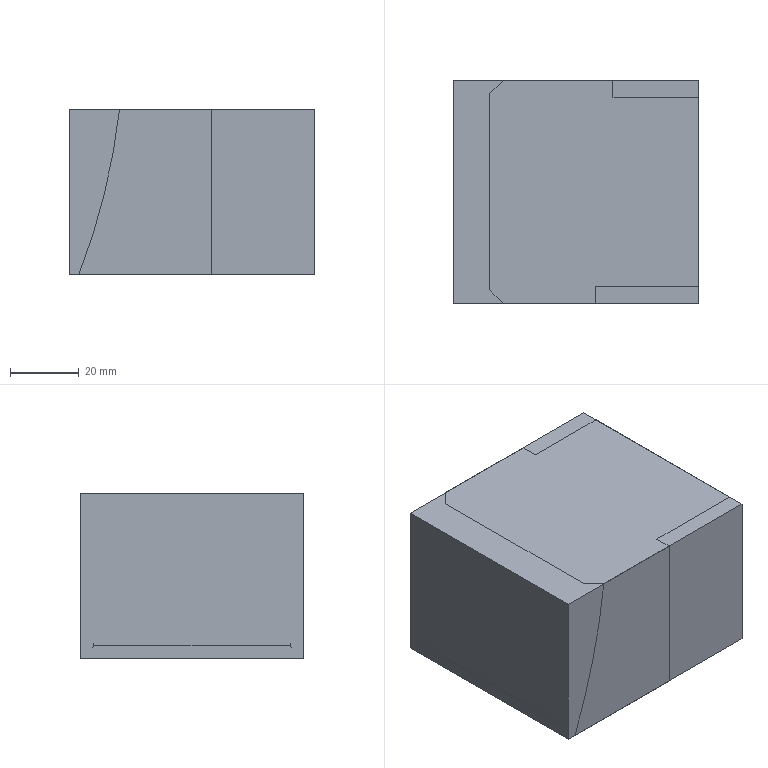Part | NX | 2 solids | 43 faces | box 71.51 x 65 x 48 mm | volume 411615 mm3 | plane 16 | cone 14 | cylinder 13 | commonest cylinder face diameters 7 x8 5 x4 379.635 x1
STEP:
#1=CARTESIAN_POINT('',(35.755,-32.5,0.));
#2=VERTEX_POINT('',#1);
#3=CARTESIAN_POINT('',(-35.755,-32.5,0.));
#4=VERTEX_POINT('',#3);
#5=CARTESIAN_POINT('',(0.,-32.5,0.));
#6=DIRECTION('',(-1.,0.,0.));
#7=VECTOR('',#6,1000.);
#8=LINE('',#5,#7);
#9=EDGE_CURVE('',#2,#4,#8,.T.);
#10=ORIENTED_EDGE('',*,*,#9,.F.);
#11=CARTESIAN_POINT('',(35.755,32.5,0.));
#12=VERTEX_POINT('',#11);
#13=CARTESIAN_POINT('',(35.755,0.,0.));
#14=DIRECTION('',(0.,-1.,0.));
#15=VECTOR('',#14,1000.);
#16=LINE('',#13,#15);
#17=EDGE_CURVE('',#12,#2,#16,.T.);
#18=ORIENTED_EDGE('',*,*,#17,.F.);
#19=CARTESIAN_POINT('',(-35.755,32.5,0.));
#20=VERTEX_POINT('',#19);
#21=CARTESIAN_POINT('',(0.,32.5,0.));
#22=DIRECTION('',(1.,0.,0.));
#23=VECTOR('',#22,1000.);
#24=LINE('',#21,#23);
#25=EDGE_CURVE('',#20,#12,#24,.T.);
#26=ORIENTED_EDGE('',*,*,#25,.F.);
#27=CARTESIAN_POINT('',(-35.755,0.,0.));
#28=DIRECTION('',(0.,1.,0.));
#29=VECTOR('',#28,1000.);
#30=LINE('',#27,#29);
#31=EDGE_CURVE('',#4,#20,#30,.T.);
#32=ORIENTED_EDGE('',*,*,#31,.F.);
#33=EDGE_LOOP('',(#10,#18,#26,#32));
#34=FACE_BOUND('',#33,.T.);
#35=CARTESIAN_POINT('',(0.,0.,0.));
#36=DIRECTION('',(0.,0.,1.));
#37=DIRECTION('',(1.,0.,0.));
#38=AXIS2_PLACEMENT_3D('',#35,#36,#37);
#39=PLANE('',#38);
#40=ADVANCED_FACE('',(#34),#39,.T.);
#41=CARTESIAN_POINT('',(35.755,-32.5,-48.));
#42=VERTEX_POINT('',#41);
#43=CARTESIAN_POINT('',(35.755,-32.5,-48.));
#44=DIRECTION('',(0.,0.,1.));
#45=VECTOR('',#44,1000.);
#46=LINE('',#43,#45);
#47=EDGE_CURVE('',#42,#2,#46,.T.);
#48=ORIENTED_EDGE('',*,*,#47,.T.);
#49=ORIENTED_EDGE('',*,*,#9,.T.);
#50=CARTESIAN_POINT('',(-35.755,-32.5,-48.));
#51=VERTEX_POINT('',#50);
#52=CARTESIAN_POINT('',(-35.755,-32.5,-48.));
#53=DIRECTION('',(0.,0.,1.));
#54=VECTOR('',#53,1000.);
#55=LINE('',#52,#54);
#56=EDGE_CURVE('',#51,#4,#55,.T.);
#57=ORIENTED_EDGE('',*,*,#56,.F.);
#58=CARTESIAN_POINT('',(0.,-32.5,-48.));
#59=DIRECTION('',(1.,0.,0.));
#60=VECTOR('',#59,1000.);
#61=LINE('',#58,#60);
#62=EDGE_CURVE('',#51,#42,#61,.T.);
#63=ORIENTED_EDGE('',*,*,#62,.T.);
#64=EDGE_LOOP('',(#48,#49,#57,#63));
#65=FACE_BOUND('',#64,.T.);
#66=CARTESIAN_POINT('',(0.,-32.5,-48.));
#67=DIRECTION('',(0.,-1.,0.));
#68=DIRECTION('',(0.,0.,-1.));
#69=AXIS2_PLACEMENT_3D('',#66,#67,#68);
#70=PLANE('',#69);
#71=ADVANCED_FACE('',(#65),#70,.T.);
#72=ORIENTED_EDGE('',*,*,#56,.T.);
#73=ORIENTED_EDGE('',*,*,#31,.T.);
#74=CARTESIAN_POINT('',(-35.755,32.5,-48.));
#75=VERTEX_POINT('',#74);
#76=CARTESIAN_POINT('',(-35.755,32.5,-48.));
#77=DIRECTION('',(0.,0.,1.));
#78=VECTOR('',#77,1000.);
#79=LINE('',#76,#78);
#80=EDGE_CURVE('',#75,#20,#79,.T.);
#81=ORIENTED_EDGE('',*,*,#80,.F.);
#82=CARTESIAN_POINT('',(-35.755,0.,-48.));
#83=DIRECTION('',(0.,-1.,0.));
#84=VECTOR('',#83,1000.);
#85=LINE('',#82,#84);
#86=EDGE_CURVE('',#75,#51,#85,.T.);
#87=ORIENTED_EDGE('',*,*,#86,.T.);
#88=EDGE_LOOP('',(#72,#73,#81,#87));
#89=FACE_BOUND('',#88,.T.);
#90=CARTESIAN_POINT('',(-35.755,0.,-48.));
#91=DIRECTION('',(-1.,0.,0.));
#92=DIRECTION('',(0.,0.,1.));
#93=AXIS2_PLACEMENT_3D('',#90,#91,#92);
#94=PLANE('',#93);
#95=ADVANCED_FACE('',(#89),#94,.T.);
#96=ORIENTED_EDGE('',*,*,#80,.T.);
#97=ORIENTED_EDGE('',*,*,#25,.T.);
#98=CARTESIAN_POINT('',(35.755,32.5,-48.));
#99=VERTEX_POINT('',#98);
#100=CARTESIAN_POINT('',(35.755,32.5,-48.));
#101=DIRECTION('',(0.,0.,1.));
#102=VECTOR('',#101,1000.);
#103=LINE('',#100,#102);
#104=EDGE_CURVE('',#99,#12,#103,.T.);
#105=ORIENTED_EDGE('',*,*,#104,.F.);
#106=CARTESIAN_POINT('',(0.,32.5,-48.));
#107=DIRECTION('',(-1.,0.,0.));
#108=VECTOR('',#107,1000.);
#109=LINE('',#106,#108);
#110=EDGE_CURVE('',#99,#75,#109,.T.);
#111=ORIENTED_EDGE('',*,*,#110,.T.);
#112=EDGE_LOOP('',(#96,#97,#105,#111));
#113=FACE_BOUND('',#112,.T.);
#114=CARTESIAN_POINT('',(0.,32.5,-48.));
#115=DIRECTION('',(0.,1.,0.));
#116=DIRECTION('',(0.,0.,1.));
#117=AXIS2_PLACEMENT_3D('',#114,#115,#116);
#118=PLANE('',#117);
#119=ADVANCED_FACE('',(#113),#118,.T.);
#120=CARTESIAN_POINT('',(35.755,0.,-48.));
#121=DIRECTION('',(0.,1.,0.));
#122=VECTOR('',#121,1000.);
#123=LINE('',#120,#122);
#124=EDGE_CURVE('',#42,#99,#123,.T.);
#125=ORIENTED_EDGE('',*,*,#124,.F.);
#126=ORIENTED_EDGE('',*,*,#62,.F.);
#127=ORIENTED_EDGE('',*,*,#86,.F.);
#128=ORIENTED_EDGE('',*,*,#110,.F.);
#129=EDGE_LOOP('',(#125,#126,#127,#128));
#130=FACE_BOUND('',#129,.T.);
#131=CARTESIAN_POINT('',(0.,0.,-48.));
#132=DIRECTION('',(0.,0.,-1.));
#133=DIRECTION('',(-1.,0.,0.));
#134=AXIS2_PLACEMENT_3D('',#131,#132,#133);
#135=PLANE('',#134);
#136=ADVANCED_FACE('',(#130),#135,.T.);
#137=ORIENTED_EDGE('',*,*,#124,.T.);
#138=ORIENTED_EDGE('',*,*,#104,.T.);
#139=ORIENTED_EDGE('',*,*,#17,.T.);
#140=ORIENTED_EDGE('',*,*,#47,.F.);
#141=EDGE_LOOP('',(#137,#138,#139,#140));
#142=FACE_BOUND('',#141,.T.);
#143=CARTESIAN_POINT('',(35.755,0.,-48.));
#144=DIRECTION('',(1.,0.,0.));
#145=DIRECTION('',(0.,0.,-1.));
#146=AXIS2_PLACEMENT_3D('',#143,#144,#145);
#147=PLANE('',#146);
#148=ADVANCED_FACE('',(#142),#147,.T.);
#149=CLOSED_SHELL('',(#40,#71,#95,#119,#136,#148));
#150=MANIFOLD_SOLID_BREP('',#149);
#151=CARTESIAN_POINT('',(23.755,-20.,-36.5));
#152=VERTEX_POINT('',#151);
#153=CARTESIAN_POINT('',(23.755,-20.,-43.5));
#154=VERTEX_POINT('',#153);
#155=CARTESIAN_POINT('',(23.755,-20.,-40.));
#156=DIRECTION('',(1.,0.,0.));
#157=DIRECTION('',(0.,0.,-1.));
#158=AXIS2_PLACEMENT_3D('',#155,#156,#157);
#159=CIRCLE('',#158,3.5);
#160=EDGE_CURVE('',#152,#154,#159,.T.);
#161=ORIENTED_EDGE('',*,*,#160,.F.);
#162=CARTESIAN_POINT('',(35.755,-20.,-36.5));
#163=VERTEX_POINT('',#162);
#164=CARTESIAN_POINT('',(35.755,-20.,-36.5));
#165=DIRECTION('',(1.,0.,0.));
#166=VECTOR('',#165,1000.);
#167=LINE('',#164,#166);
#168=EDGE_CURVE('',#163,#152,#167,.F.);
#169=ORIENTED_EDGE('',*,*,#168,.F.);
#170=CARTESIAN_POINT('',(35.755,-20.,-43.5));
#171=VERTEX_POINT('',#170);
#172=CARTESIAN_POINT('',(35.755,-20.,-40.));
#173=DIRECTION('',(1.,0.,0.));
#174=DIRECTION('',(0.,0.,-1.));
#175=AXIS2_PLACEMENT_3D('',#172,#173,#174);
#176=CIRCLE('',#175,3.5);
#177=EDGE_CURVE('',#163,#171,#176,.T.);
#178=ORIENTED_EDGE('',*,*,#177,.T.);
#179=CARTESIAN_POINT('',(35.755,-20.,-43.5));
#180=DIRECTION('',(1.,0.,0.));
#181=VECTOR('',#180,1000.);
#182=LINE('',#179,#181);
#183=EDGE_CURVE('',#171,#154,#182,.F.);
#184=ORIENTED_EDGE('',*,*,#183,.T.);
#185=EDGE_LOOP('',(#161,#169,#178,#184));
#186=FACE_BOUND('',#185,.T.);
#187=CARTESIAN_POINT('',(35.755,-20.,-40.));
#188=DIRECTION('',(1.,0.,0.));
#189=DIRECTION('',(0.,0.,1.));
#190=AXIS2_PLACEMENT_3D('',#187,#188,#189);
#191=CYLINDRICAL_SURFACE('',#190,3.5);
#192=ADVANCED_FACE('',(#186),#191,.F.);
#193=CARTESIAN_POINT('',(21.652,-20.,-40.));
#194=VERTEX_POINT('',#193);
#195=CARTESIAN_POINT('',(23.755,-20.,-43.5));
#196=DIRECTION('',(0.515,0.,-0.8572));
#197=VECTOR('',#196,1000.);
#198=LINE('',#195,#197);
#199=EDGE_CURVE('',#154,#194,#198,.F.);
#200=ORIENTED_EDGE('',*,*,#199,.T.);
#201=CARTESIAN_POINT('',(23.755,-20.,-36.5));
#202=DIRECTION('',(0.515,0.,0.8572));
#203=VECTOR('',#202,1000.);
#204=LINE('',#201,#203);
#205=EDGE_CURVE('',#152,#194,#204,.F.);
#206=ORIENTED_EDGE('',*,*,#205,.F.);
#207=ORIENTED_EDGE('',*,*,#160,.T.);
#208=EDGE_LOOP('',(#200,#206,#207));
#209=FACE_BOUND('',#208,.T.);
#210=CARTESIAN_POINT('',(23.755,-20.,-40.));
#211=DIRECTION('',(1.,0.,0.));
#212=DIRECTION('',(0.,0.,1.));
#213=AXIS2_PLACEMENT_3D('',#210,#211,#212);
#214=CONICAL_SURFACE('',#213,3.5,1.03);
#215=ADVANCED_FACE('',(#209),#214,.F.);
#216=CARTESIAN_POINT('',(23.755,-20.,-4.5));
#217=VERTEX_POINT('',#216);
#218=CARTESIAN_POINT('',(23.755,-20.,-11.5));
#219=VERTEX_POINT('',#218);
#220=CARTESIAN_POINT('',(23.755,-20.,-8.));
#221=DIRECTION('',(1.,0.,0.));
#222=DIRECTION('',(0.,0.,-1.));
#223=AXIS2_PLACEMENT_3D('',#220,#221,#222);
#224=CIRCLE('',#223,3.5);
#225=EDGE_CURVE('',#217,#219,#224,.T.);
#226=ORIENTED_EDGE('',*,*,#225,.F.);
#227=CARTESIAN_POINT('',(35.755,-20.,-4.5));
#228=VERTEX_POINT('',#227);
#229=CARTESIAN_POINT('',(35.755,-20.,-4.5));
#230=DIRECTION('',(1.,0.,0.));
#231=VECTOR('',#230,1000.);
#232=LINE('',#229,#231);
#233=EDGE_CURVE('',#228,#217,#232,.F.);
#234=ORIENTED_EDGE('',*,*,#233,.F.);
#235=CARTESIAN_POINT('',(35.755,-20.,-11.5));
#236=VERTEX_POINT('',#235);
#237=CARTESIAN_POINT('',(35.755,-20.,-8.));
#238=DIRECTION('',(1.,0.,0.));
#239=DIRECTION('',(0.,0.,-1.));
#240=AXIS2_PLACEMENT_3D('',#237,#238,#239);
#241=CIRCLE('',#240,3.5);
#242=EDGE_CURVE('',#228,#236,#241,.T.);
#243=ORIENTED_EDGE('',*,*,#242,.T.);
#244=CARTESIAN_POINT('',(35.755,-20.,-11.5));
#245=DIRECTION('',(1.,0.,0.));
#246=VECTOR('',#245,1000.);
#247=LINE('',#244,#246);
#248=EDGE_CURVE('',#236,#219,#247,.F.);
#249=ORIENTED_EDGE('',*,*,#248,.T.);
#250=EDGE_LOOP('',(#226,#234,#243,#249));
#251=FACE_BOUND('',#250,.T.);
#252=CARTESIAN_POINT('',(35.755,-20.,-8.));
#253=DIRECTION('',(1.,0.,0.));
#254=DIRECTION('',(0.,0.,1.));
#255=AXIS2_PLACEMENT_3D('',#252,#253,#254);
#256=CYLINDRICAL_SURFACE('',#255,3.5);
#257=ADVANCED_FACE('',(#251),#256,.F.);
#258=CARTESIAN_POINT('',(21.652,-20.,-8.));
#259=VERTEX_POINT('',#258);
#260=CARTESIAN_POINT('',(23.755,-20.,-11.5));
#261=DIRECTION('',(0.515,0.,-0.8572));
#262=VECTOR('',#261,1000.);
#263=LINE('',#260,#262);
#264=EDGE_CURVE('',#219,#259,#263,.F.);
#265=ORIENTED_EDGE('',*,*,#264,.T.);
#266=CARTESIAN_POINT('',(23.755,-20.,-4.5));
#267=DIRECTION('',(0.515,0.,0.8572));
#268=VECTOR('',#267,1000.);
#269=LINE('',#266,#268);
#270=EDGE_CURVE('',#217,#259,#269,.F.);
#271=ORIENTED_EDGE('',*,*,#270,.F.);
#272=ORIENTED_EDGE('',*,*,#225,.T.);
#273=EDGE_LOOP('',(#265,#271,#272));
#274=FACE_BOUND('',#273,.T.);
#275=CARTESIAN_POINT('',(23.755,-20.,-8.));
#276=DIRECTION('',(1.,0.,0.));
#277=DIRECTION('',(0.,0.,1.));
#278=AXIS2_PLACEMENT_3D('',#275,#276,#277);
#279=CONICAL_SURFACE('',#278,3.5,1.03);
#280=ADVANCED_FACE('',(#274),#279,.F.);
#281=CARTESIAN_POINT('',(23.755,20.,-4.5));
#282=VERTEX_POINT('',#281);
#283=CARTESIAN_POINT('',(23.755,20.,-11.5));
#284=VERTEX_POINT('',#283);
#285=CARTESIAN_POINT('',(23.755,20.,-8.));
#286=DIRECTION('',(1.,0.,0.));
#287=DIRECTION('',(0.,0.,-1.));
#288=AXIS2_PLACEMENT_3D('',#285,#286,#287);
#289=CIRCLE('',#288,3.5);
#290=EDGE_CURVE('',#282,#284,#289,.T.);
#291=ORIENTED_EDGE('',*,*,#290,.F.);
#292=CARTESIAN_POINT('',(35.755,20.,-4.5));
#293=VERTEX_POINT('',#292);
#294=CARTESIAN_POINT('',(35.755,20.,-4.5));
#295=DIRECTION('',(1.,0.,0.));
#296=VECTOR('',#295,1000.);
#297=LINE('',#294,#296);
#298=EDGE_CURVE('',#293,#282,#297,.F.);
#299=ORIENTED_EDGE('',*,*,#298,.F.);
#300=CARTESIAN_POINT('',(35.755,20.,-11.5));
#301=VERTEX_POINT('',#300);
#302=CARTESIAN_POINT('',(35.755,20.,-8.));
#303=DIRECTION('',(1.,0.,0.));
#304=DIRECTION('',(0.,0.,-1.));
#305=AXIS2_PLACEMENT_3D('',#302,#303,#304);
#306=CIRCLE('',#305,3.5);
#307=EDGE_CURVE('',#293,#301,#306,.T.);
#308=ORIENTED_EDGE('',*,*,#307,.T.);
#309=CARTESIAN_POINT('',(35.755,20.,-11.5));
#310=DIRECTION('',(1.,0.,0.));
#311=VECTOR('',#310,1000.);
#312=LINE('',#309,#311);
#313=EDGE_CURVE('',#301,#284,#312,.F.);
#314=ORIENTED_EDGE('',*,*,#313,.T.);
#315=EDGE_LOOP('',(#291,#299,#308,#314));
#316=FACE_BOUND('',#315,.T.);
#317=CARTESIAN_POINT('',(35.755,20.,-8.));
#318=DIRECTION('',(1.,0.,0.));
#319=DIRECTION('',(0.,0.,1.));
#320=AXIS2_PLACEMENT_3D('',#317,#318,#319);
#321=CYLINDRICAL_SURFACE('',#320,3.5);
#322=ADVANCED_FACE('',(#316),#321,.F.);
#323=CARTESIAN_POINT('',(21.652,20.,-8.));
#324=VERTEX_POINT('',#323);
#325=CARTESIAN_POINT('',(23.755,20.,-11.5));
#326=DIRECTION('',(0.515,0.,-0.8572));
#327=VECTOR('',#326,1000.);
#328=LINE('',#325,#327);
#329=EDGE_CURVE('',#284,#324,#328,.F.);
#330=ORIENTED_EDGE('',*,*,#329,.T.);
#331=CARTESIAN_POINT('',(23.755,20.,-4.5));
#332=DIRECTION('',(0.515,0.,0.8572));
#333=VECTOR('',#332,1000.);
#334=LINE('',#331,#333);
#335=EDGE_CURVE('',#282,#324,#334,.F.);
#336=ORIENTED_EDGE('',*,*,#335,.F.);
#337=ORIENTED_EDGE('',*,*,#290,.T.);
#338=EDGE_LOOP('',(#330,#336,#337));
#339=FACE_BOUND('',#338,.T.);
#340=CARTESIAN_POINT('',(23.755,20.,-8.));
#341=DIRECTION('',(1.,0.,0.));
#342=DIRECTION('',(0.,0.,1.));
#343=AXIS2_PLACEMENT_3D('',#340,#341,#342);
#344=CONICAL_SURFACE('',#343,3.5,1.03);
#345=ADVANCED_FACE('',(#339),#344,.F.);
#346=CARTESIAN_POINT('',(23.755,20.,-36.5));
#347=VERTEX_POINT('',#346);
#348=CARTESIAN_POINT('',(23.755,20.,-43.5));
#349=VERTEX_POINT('',#348);
#350=CARTESIAN_POINT('',(23.755,20.,-40.));
#351=DIRECTION('',(1.,0.,0.));
#352=DIRECTION('',(0.,0.,-1.));
#353=AXIS2_PLACEMENT_3D('',#350,#351,#352);
#354=CIRCLE('',#353,3.5);
#355=EDGE_CURVE('',#347,#349,#354,.T.);
#356=ORIENTED_EDGE('',*,*,#355,.F.);
#357=CARTESIAN_POINT('',(35.755,20.,-36.5));
#358=VERTEX_POINT('',#357);
#359=CARTESIAN_POINT('',(35.755,20.,-36.5));
#360=DIRECTION('',(1.,0.,0.));
#361=VECTOR('',#360,1000.);
#362=LINE('',#359,#361);
#363=EDGE_CURVE('',#358,#347,#362,.F.);
#364=ORIENTED_EDGE('',*,*,#363,.F.);
#365=CARTESIAN_POINT('',(35.755,20.,-43.5));
#366=VERTEX_POINT('',#365);
#367=CARTESIAN_POINT('',(35.755,20.,-40.));
#368=DIRECTION('',(1.,0.,0.));
#369=DIRECTION('',(0.,0.,-1.));
#370=AXIS2_PLACEMENT_3D('',#367,#368,#369);
#371=CIRCLE('',#370,3.5);
#372=EDGE_CURVE('',#358,#366,#371,.T.);
#373=ORIENTED_EDGE('',*,*,#372,.T.);
#374=CARTESIAN_POINT('',(35.755,20.,-43.5));
#375=DIRECTION('',(1.,0.,0.));
#376=VECTOR('',#375,1000.);
#377=LINE('',#374,#376);
#378=EDGE_CURVE('',#366,#349,#377,.F.);
#379=ORIENTED_EDGE('',*,*,#378,.T.);
#380=EDGE_LOOP('',(#356,#364,#373,#379));
#381=FACE_BOUND('',#380,.T.);
#382=CARTESIAN_POINT('',(35.755,20.,-40.));
#383=DIRECTION('',(1.,0.,0.));
#384=DIRECTION('',(0.,0.,1.));
#385=AXIS2_PLACEMENT_3D('',#382,#383,#384);
#386=CYLINDRICAL_SURFACE('',#385,3.5);
#387=ADVANCED_FACE('',(#381),#386,.F.);
#388=CARTESIAN_POINT('',(21.652,20.,-40.));
#389=VERTEX_POINT('',#388);
#390=CARTESIAN_POINT('',(23.755,20.,-43.5));
#391=DIRECTION('',(0.515,0.,-0.8572));
#392=VECTOR('',#391,1000.);
#393=LINE('',#390,#392);
#394=EDGE_CURVE('',#349,#389,#393,.F.);
#395=ORIENTED_EDGE('',*,*,#394,.T.);
#396=CARTESIAN_POINT('',(23.755,20.,-36.5));
#397=DIRECTION('',(0.515,0.,0.8572));
#398=VECTOR('',#397,1000.);
#399=LINE('',#396,#398);
#400=EDGE_CURVE('',#347,#389,#399,.F.);
#401=ORIENTED_EDGE('',*,*,#400,.F.);
#402=ORIENTED_EDGE('',*,*,#355,.T.);
#403=EDGE_LOOP('',(#395,#401,#402));
#404=FACE_BOUND('',#403,.T.);
#405=CARTESIAN_POINT('',(23.755,20.,-40.));
#406=DIRECTION('',(1.,0.,0.));
#407=DIRECTION('',(0.,0.,1.));
#408=AXIS2_PLACEMENT_3D('',#405,#406,#407);
#409=CONICAL_SURFACE('',#408,3.5,1.03);
#410=ADVANCED_FACE('',(#404),#409,.F.);
#411=CARTESIAN_POINT('',(23.755,-20.,-21.5));
#412=VERTEX_POINT('',#411);
#413=CARTESIAN_POINT('',(23.755,-20.,-26.5));
#414=VERTEX_POINT('',#413);
#415=CARTESIAN_POINT('',(23.755,-20.,-24.));
#416=DIRECTION('',(1.,0.,0.));
#417=DIRECTION('',(0.,0.,-1.));
#418=AXIS2_PLACEMENT_3D('',#415,#416,#417);
#419=CIRCLE('',#418,2.5);
#420=EDGE_CURVE('',#412,#414,#419,.T.);
#421=ORIENTED_EDGE('',*,*,#420,.F.);
#422=CARTESIAN_POINT('',(35.755,-20.,-21.5));
#423=VERTEX_POINT('',#422);
#424=CARTESIAN_POINT('',(35.755,-20.,-21.5));
#425=DIRECTION('',(1.,0.,0.));
#426=VECTOR('',#425,1000.);
#427=LINE('',#424,#426);
#428=EDGE_CURVE('',#423,#412,#427,.F.);
#429=ORIENTED_EDGE('',*,*,#428,.F.);
#430=CARTESIAN_POINT('',(35.755,-20.,-26.5));
#431=VERTEX_POINT('',#430);
#432=CARTESIAN_POINT('',(35.755,-20.,-24.));
#433=DIRECTION('',(1.,0.,0.));
#434=DIRECTION('',(0.,0.,-1.));
#435=AXIS2_PLACEMENT_3D('',#432,#433,#434);
#436=CIRCLE('',#435,2.5);
#437=EDGE_CURVE('',#423,#431,#436,.T.);
#438=ORIENTED_EDGE('',*,*,#437,.T.);
#439=CARTESIAN_POINT('',(35.755,-20.,-26.5));
#440=DIRECTION('',(1.,0.,0.));
#441=VECTOR('',#440,1000.);
#442=LINE('',#439,#441);
#443=EDGE_CURVE('',#431,#414,#442,.F.);
#444=ORIENTED_EDGE('',*,*,#443,.T.);
#445=EDGE_LOOP('',(#421,#429,#438,#444));
#446=FACE_BOUND('',#445,.T.);
#447=CARTESIAN_POINT('',(35.755,-20.,-24.));
#448=DIRECTION('',(1.,0.,0.));
#449=DIRECTION('',(0.,0.,1.));
#450=AXIS2_PLACEMENT_3D('',#447,#448,#449);
#451=CYLINDRICAL_SURFACE('',#450,2.5);
#452=ADVANCED_FACE('',(#446),#451,.F.);
#453=CARTESIAN_POINT('',(22.253,-20.,-24.));
#454=VERTEX_POINT('',#453);
#455=CARTESIAN_POINT('',(23.755,-20.,-26.5));
#456=DIRECTION('',(0.515,0.,-0.8572));
#457=VECTOR('',#456,1000.);
#458=LINE('',#455,#457);
#459=EDGE_CURVE('',#414,#454,#458,.F.);
#460=ORIENTED_EDGE('',*,*,#459,.T.);
#461=CARTESIAN_POINT('',(23.755,-20.,-21.5));
#462=DIRECTION('',(0.515,0.,0.8572));
#463=VECTOR('',#462,1000.);
#464=LINE('',#461,#463);
#465=EDGE_CURVE('',#412,#454,#464,.F.);
#466=ORIENTED_EDGE('',*,*,#465,.F.);
#467=ORIENTED_EDGE('',*,*,#420,.T.);
#468=EDGE_LOOP('',(#460,#466,#467));
#469=FACE_BOUND('',#468,.T.);
#470=CARTESIAN_POINT('',(23.755,-20.,-24.));
#471=DIRECTION('',(1.,0.,0.));
#472=DIRECTION('',(0.,0.,1.));
#473=AXIS2_PLACEMENT_3D('',#470,#471,#472);
#474=CONICAL_SURFACE('',#473,2.5,1.03);
#475=ADVANCED_FACE('',(#469),#474,.F.);
#476=CARTESIAN_POINT('',(23.755,20.,-21.5));
#477=VERTEX_POINT('',#476);
#478=CARTESIAN_POINT('',(23.755,20.,-26.5));
#479=VERTEX_POINT('',#478);
#480=CARTESIAN_POINT('',(23.755,20.,-24.));
#481=DIRECTION('',(1.,0.,0.));
#482=DIRECTION('',(0.,0.,-1.));
#483=AXIS2_PLACEMENT_3D('',#480,#481,#482);
#484=CIRCLE('',#483,2.5);
#485=EDGE_CURVE('',#477,#479,#484,.T.);
#486=ORIENTED_EDGE('',*,*,#485,.F.);
#487=CARTESIAN_POINT('',(35.755,20.,-21.5));
#488=VERTEX_POINT('',#487);
#489=CARTESIAN_POINT('',(35.755,20.,-21.5));
#490=DIRECTION('',(1.,0.,0.));
#491=VECTOR('',#490,1000.);
#492=LINE('',#489,#491);
#493=EDGE_CURVE('',#488,#477,#492,.F.);
#494=ORIENTED_EDGE('',*,*,#493,.F.);
#495=CARTESIAN_POINT('',(35.755,20.,-26.5));
#496=VERTEX_POINT('',#495);
#497=CARTESIAN_POINT('',(35.755,20.,-24.));
#498=DIRECTION('',(1.,0.,0.));
#499=DIRECTION('',(0.,0.,-1.));
#500=AXIS2_PLACEMENT_3D('',#497,#498,#499);
#501=CIRCLE('',#500,2.5);
#502=EDGE_CURVE('',#488,#496,#501,.T.);
#503=ORIENTED_EDGE('',*,*,#502,.T.);
#504=CARTESIAN_POINT('',(35.755,20.,-26.5));
#505=DIRECTION('',(1.,0.,0.));
#506=VECTOR('',#505,1000.);
#507=LINE('',#504,#506);
#508=EDGE_CURVE('',#496,#479,#507,.F.);
#509=ORIENTED_EDGE('',*,*,#508,.T.);
#510=EDGE_LOOP('',(#486,#494,#503,#509));
#511=FACE_BOUND('',#510,.T.);
#512=CARTESIAN_POINT('',(35.755,20.,-24.));
#513=DIRECTION('',(1.,0.,0.));
#514=DIRECTION('',(0.,0.,1.));
#515=AXIS2_PLACEMENT_3D('',#512,#513,#514);
#516=CYLINDRICAL_SURFACE('',#515,2.5);
#517=ADVANCED_FACE('',(#511),#516,.F.);
#518=CARTESIAN_POINT('',(22.253,20.,-24.));
#519=VERTEX_POINT('',#518);
#520=CARTESIAN_POINT('',(23.755,20.,-26.5));
#521=DIRECTION('',(0.515,0.,-0.8572));
#522=VECTOR('',#521,1000.);
#523=LINE('',#520,#522);
#524=EDGE_CURVE('',#479,#519,#523,.F.);
#525=ORIENTED_EDGE('',*,*,#524,.T.);
#526=CARTESIAN_POINT('',(23.755,20.,-21.5));
#527=DIRECTION('',(0.515,0.,0.8572));
#528=VECTOR('',#527,1000.);
#529=LINE('',#526,#528);
#530=EDGE_CURVE('',#477,#519,#529,.F.);
#531=ORIENTED_EDGE('',*,*,#530,.F.);
#532=ORIENTED_EDGE('',*,*,#485,.T.);
#533=EDGE_LOOP('',(#525,#531,#532));
#534=FACE_BOUND('',#533,.T.);
#535=CARTESIAN_POINT('',(23.755,20.,-24.));
#536=DIRECTION('',(1.,0.,0.));
#537=DIRECTION('',(0.,0.,1.));
#538=AXIS2_PLACEMENT_3D('',#535,#536,#537);
#539=CONICAL_SURFACE('',#538,2.5,1.03);
#540=ADVANCED_FACE('',(#534),#539,.F.);
#541=CARTESIAN_POINT('',(35.755,20.,-24.));
#542=DIRECTION('',(1.,0.,0.));
#543=DIRECTION('',(0.,0.,-1.));
#544=AXIS2_PLACEMENT_3D('',#541,#542,#543);
#545=CIRCLE('',#544,2.5);
#546=EDGE_CURVE('',#496,#488,#545,.T.);
#547=ORIENTED_EDGE('',*,*,#546,.F.);
#548=ORIENTED_EDGE('',*,*,#502,.F.);
#549=EDGE_LOOP('',(#547,#548));
#550=FACE_BOUND('',#549,.T.);
#551=CARTESIAN_POINT('',(35.755,-20.,-24.));
#552=DIRECTION('',(1.,0.,0.));
#553=DIRECTION('',(0.,0.,-1.));
#554=AXIS2_PLACEMENT_3D('',#551,#552,#553);
#555=CIRCLE('',#554,2.5);
#556=EDGE_CURVE('',#431,#423,#555,.T.);
#557=ORIENTED_EDGE('',*,*,#556,.F.);
#558=ORIENTED_EDGE('',*,*,#437,.F.);
#559=EDGE_LOOP('',(#557,#558));
#560=FACE_BOUND('',#559,.T.);
#561=CARTESIAN_POINT('',(35.755,20.,-40.));
#562=DIRECTION('',(1.,0.,0.));
#563=DIRECTION('',(0.,0.,-1.));
#564=AXIS2_PLACEMENT_3D('',#561,#562,#563);
#565=CIRCLE('',#564,3.5);
#566=EDGE_CURVE('',#366,#358,#565,.T.);
#567=ORIENTED_EDGE('',*,*,#566,.F.);
#568=ORIENTED_EDGE('',*,*,#372,.F.);
#569=EDGE_LOOP('',(#567,#568));
#570=FACE_BOUND('',#569,.T.);
#571=CARTESIAN_POINT('',(35.755,20.,-8.));
#572=DIRECTION('',(1.,0.,0.));
#573=DIRECTION('',(0.,0.,-1.));
#574=AXIS2_PLACEMENT_3D('',#571,#572,#573);
#575=CIRCLE('',#574,3.5);
#576=EDGE_CURVE('',#301,#293,#575,.T.);
#577=ORIENTED_EDGE('',*,*,#576,.F.);
#578=ORIENTED_EDGE('',*,*,#307,.F.);
#579=EDGE_LOOP('',(#577,#578));
#580=FACE_BOUND('',#579,.T.);
#581=CARTESIAN_POINT('',(35.755,-20.,-8.));
#582=DIRECTION('',(1.,0.,0.));
#583=DIRECTION('',(0.,0.,-1.));
#584=AXIS2_PLACEMENT_3D('',#581,#582,#583);
#585=CIRCLE('',#584,3.5);
#586=EDGE_CURVE('',#236,#228,#585,.T.);
#587=ORIENTED_EDGE('',*,*,#586,.F.);
#588=ORIENTED_EDGE('',*,*,#242,.F.);
#589=EDGE_LOOP('',(#587,#588));
#590=FACE_BOUND('',#589,.T.);
#591=CARTESIAN_POINT('',(35.755,-20.,-40.));
#592=DIRECTION('',(1.,0.,0.));
#593=DIRECTION('',(0.,0.,-1.));
#594=AXIS2_PLACEMENT_3D('',#591,#592,#593);
#595=CIRCLE('',#594,3.5);
#596=EDGE_CURVE('',#171,#163,#595,.T.);
#597=ORIENTED_EDGE('',*,*,#596,.F.);
#598=ORIENTED_EDGE('',*,*,#177,.F.);
#599=EDGE_LOOP('',(#597,#598));
#600=FACE_BOUND('',#599,.T.);
#601=CARTESIAN_POINT('',(35.755,27.5,0.));
#602=VERTEX_POINT('',#601);
#603=CARTESIAN_POINT('',(35.755,27.5,-48.));
#604=VERTEX_POINT('',#603);
#605=CARTESIAN_POINT('',(35.755,27.5,-48.));
#606=DIRECTION('',(0.,0.,-1.));
#607=VECTOR('',#606,1000.);
#608=LINE('',#605,#607);
#609=EDGE_CURVE('',#602,#604,#608,.T.);
#610=ORIENTED_EDGE('',*,*,#609,.F.);
#611=CARTESIAN_POINT('',(35.755,-27.5,0.));
#612=VERTEX_POINT('',#611);
#613=CARTESIAN_POINT('',(35.755,-32.5,0.));
#614=DIRECTION('',(0.,-1.,0.));
#615=VECTOR('',#614,1000.);
#616=LINE('',#613,#615);
#617=EDGE_CURVE('',#602,#612,#616,.T.);
#618=ORIENTED_EDGE('',*,*,#617,.T.);
#619=CARTESIAN_POINT('',(35.755,-27.5,-48.));
#620=VERTEX_POINT('',#619);
#621=CARTESIAN_POINT('',(35.755,-27.5,-48.));
#622=DIRECTION('',(0.,0.,1.));
#623=VECTOR('',#622,1000.);
#624=LINE('',#621,#623);
#625=EDGE_CURVE('',#620,#612,#624,.T.);
#626=ORIENTED_EDGE('',*,*,#625,.F.);
#627=CARTESIAN_POINT('',(35.755,-32.5,-48.));
#628=DIRECTION('',(0.,-1.,0.));
#629=VECTOR('',#628,1000.);
#630=LINE('',#627,#629);
#631=EDGE_CURVE('',#604,#620,#630,.T.);
#632=ORIENTED_EDGE('',*,*,#631,.F.);
#633=EDGE_LOOP('',(#610,#618,#626,#632));
#634=FACE_BOUND('',#633,.T.);
#635=CARTESIAN_POINT('',(35.755,-32.5,-48.));
#636=DIRECTION('',(-1.,0.,0.));
#637=DIRECTION('',(0.,0.,-1.));
#638=AXIS2_PLACEMENT_3D('',#635,#636,#637);
#639=PLANE('',#638);
#640=ADVANCED_FACE('',(#550,#560,#570,#580,#590,#600,#634),#639,.F.);
#641=CARTESIAN_POINT('',(-34.125,-31.367,-48.));
#642=VERTEX_POINT('',#641);
#643=CARTESIAN_POINT('',(-35.755,-28.5,-44.226));
#644=VERTEX_POINT('',#643);
#645=CARTESIAN_POINT('',(-34.125,-31.367,-48.));
#646=CARTESIAN_POINT('',(-34.667,-30.406,-46.745));
#647=CARTESIAN_POINT('',(-35.21,-29.451,-45.487));
#648=CARTESIAN_POINT('',(-35.755,-28.5,-44.226));
#649=B_SPLINE_CURVE_WITH_KNOTS('',3,(#645,#646,#647,#648),.UNSPECIFIED.,.F.,.F.,(4,4),(0.,1.),.PIECEWISE_BEZIER_KNOTS.);
#650=EDGE_CURVE('',#642,#644,#649,.T.);
#651=ORIENTED_EDGE('',*,*,#650,.T.);
#652=CARTESIAN_POINT('',(-35.755,28.5,-44.226));
#653=VERTEX_POINT('',#652);
#654=CARTESIAN_POINT('',(-35.755,122.5,-44.226));
#655=DIRECTION('',(0.,-1.,0.));
#656=VECTOR('',#655,1000.);
#657=LINE('',#654,#656);
#658=EDGE_CURVE('',#653,#644,#657,.T.);
#659=ORIENTED_EDGE('',*,*,#658,.F.);
#660=CARTESIAN_POINT('',(-34.125,31.367,-48.));
#661=VERTEX_POINT('',#660);
#662=CARTESIAN_POINT('',(-35.755,28.5,-44.226));
#663=CARTESIAN_POINT('',(-35.21,29.451,-45.487));
#664=CARTESIAN_POINT('',(-34.667,30.406,-46.745));
#665=CARTESIAN_POINT('',(-34.125,31.367,-48.));
#666=B_SPLINE_CURVE_WITH_KNOTS('',3,(#662,#663,#664,#665),.UNSPECIFIED.,.F.,.F.,(4,4),(0.,1.),.PIECEWISE_BEZIER_KNOTS.);
#667=EDGE_CURVE('',#653,#661,#666,.T.);
#668=ORIENTED_EDGE('',*,*,#667,.T.);
#669=CARTESIAN_POINT('',(-34.125,0.,-48.));
#670=DIRECTION('',(0.,1.,0.));
#671=VECTOR('',#670,1000.);
#672=LINE('',#669,#671);
#673=EDGE_CURVE('',#642,#661,#672,.T.);
#674=ORIENTED_EDGE('',*,*,#673,.F.);
#675=EDGE_LOOP('',(#651,#659,#668,#674));
#676=FACE_BOUND('',#675,.T.);
#677=CARTESIAN_POINT('',(-34.125,122.5,-48.));
#678=DIRECTION('',(-0.918,0.,-0.3965));
#679=DIRECTION('',(0.,1.,0.));
#680=AXIS2_PLACEMENT_3D('',#677,#678,#679);
#681=PLANE('',#680);
#682=ADVANCED_FACE('',(#676),#681,.T.);
#683=CARTESIAN_POINT('',(-32.91,32.5,-48.));
#684=VERTEX_POINT('',#683);
#685=CARTESIAN_POINT('',(10.755,32.5,-48.));
#686=VERTEX_POINT('',#685);
#687=CARTESIAN_POINT('',(-39.245,32.5,-48.));
#688=DIRECTION('',(1.,0.,0.));
#689=VECTOR('',#688,1000.);
#690=LINE('',#687,#689);
#691=EDGE_CURVE('',#684,#686,#690,.T.);
#692=ORIENTED_EDGE('',*,*,#691,.T.);
#693=CARTESIAN_POINT('',(10.755,27.5,-48.));
#694=VERTEX_POINT('',#693);
#695=CARTESIAN_POINT('',(10.755,27.5,-48.));
#696=DIRECTION('',(0.,1.,0.));
#697=VECTOR('',#696,1000.);
#698=LINE('',#695,#697);
#699=EDGE_CURVE('',#694,#686,#698,.T.);
#700=ORIENTED_EDGE('',*,*,#699,.F.);
#701=CARTESIAN_POINT('',(35.755,27.5,-48.));
#702=DIRECTION('',(-1.,0.,0.));
#703=VECTOR('',#702,1000.);
#704=LINE('',#701,#703);
#705=EDGE_CURVE('',#604,#694,#704,.T.);
#706=ORIENTED_EDGE('',*,*,#705,.F.);
#707=ORIENTED_EDGE('',*,*,#631,.T.);
#708=CARTESIAN_POINT('',(5.755,-27.5,-48.));
#709=VERTEX_POINT('',#708);
#710=CARTESIAN_POINT('',(35.755,-27.5,-48.));
#711=DIRECTION('',(1.,0.,0.));
#712=VECTOR('',#711,1000.);
#713=LINE('',#710,#712);
#714=EDGE_CURVE('',#709,#620,#713,.T.);
#715=ORIENTED_EDGE('',*,*,#714,.F.);
#716=CARTESIAN_POINT('',(5.755,-32.5,-48.));
#717=VERTEX_POINT('',#716);
#718=CARTESIAN_POINT('',(5.755,-27.5,-48.));
#719=DIRECTION('',(0.,-1.,0.));
#720=VECTOR('',#719,1000.);
#721=LINE('',#718,#720);
#722=EDGE_CURVE('',#709,#717,#721,.T.);
#723=ORIENTED_EDGE('',*,*,#722,.T.);
#724=CARTESIAN_POINT('',(-32.91,-32.5,-48.));
#725=VERTEX_POINT('',#724);
#726=CARTESIAN_POINT('',(-39.245,-32.5,-48.));
#727=DIRECTION('',(-1.,0.,0.));
#728=VECTOR('',#727,1000.);
#729=LINE('',#726,#728);
#730=EDGE_CURVE('',#717,#725,#729,.T.);
#731=ORIENTED_EDGE('',*,*,#730,.T.);
#732=CARTESIAN_POINT('',(-32.91,-32.5,-48.));
#733=CARTESIAN_POINT('',(-33.315,-32.122,-48.));
#734=CARTESIAN_POINT('',(-33.72,-31.745,-48.));
#735=CARTESIAN_POINT('',(-34.125,-31.367,-48.));
#736=B_SPLINE_CURVE_WITH_KNOTS('',3,(#732,#733,#734,#735),.UNSPECIFIED.,.F.,.F.,(4,4),(0.,1.),.PIECEWISE_BEZIER_KNOTS.);
#737=EDGE_CURVE('',#725,#642,#736,.T.);
#738=ORIENTED_EDGE('',*,*,#737,.T.);
#739=ORIENTED_EDGE('',*,*,#673,.T.);
#740=CARTESIAN_POINT('',(-34.125,31.367,-48.));
#741=CARTESIAN_POINT('',(-33.72,31.745,-48.));
#742=CARTESIAN_POINT('',(-33.315,32.122,-48.));
#743=CARTESIAN_POINT('',(-32.91,32.5,-48.));
#744=B_SPLINE_CURVE_WITH_KNOTS('',3,(#740,#741,#742,#743),.UNSPECIFIED.,.F.,.F.,(4,4),(0.,1.),.PIECEWISE_BEZIER_KNOTS.);
#745=EDGE_CURVE('',#661,#684,#744,.T.);
#746=ORIENTED_EDGE('',*,*,#745,.T.);
#747=EDGE_LOOP('',(#692,#700,#706,#707,#715,#723,#731,#738,#739,#746));
#748=FACE_BOUND('',#747,.T.);
#749=CARTESIAN_POINT('',(-1.745,0.,-48.));
#750=DIRECTION('',(0.,0.,1.));
#751=DIRECTION('',(0.,1.,0.));
#752=AXIS2_PLACEMENT_3D('',#749,#750,#751);
#753=PLANE('',#752);
#754=ADVANCED_FACE('',(#748),#753,.F.);
#755=CARTESIAN_POINT('',(-21.08,32.5,0.));
#756=VERTEX_POINT('',#755);
#757=CARTESIAN_POINT('',(-25.107,28.5,0.));
#758=VERTEX_POINT('',#757);
#759=CARTESIAN_POINT('',(-21.08,32.5,0.));
#760=CARTESIAN_POINT('',(-22.422,31.167,0.));
#761=CARTESIAN_POINT('',(-23.764,29.833,0.));
#762=CARTESIAN_POINT('',(-25.107,28.5,0.));
#763=B_SPLINE_CURVE_WITH_KNOTS('',3,(#759,#760,#761,#762),.UNSPECIFIED.,.F.,.F.,(4,4),(0.,1.),.PIECEWISE_BEZIER_KNOTS.);
#764=EDGE_CURVE('',#756,#758,#763,.T.);
#765=ORIENTED_EDGE('',*,*,#764,.F.);
#766=CARTESIAN_POINT('',(-213.645,32.5,22.));
#767=DIRECTION('',(0.,-1.,0.));
#768=DIRECTION('',(0.,0.,-1.));
#769=AXIS2_PLACEMENT_3D('',#766,#767,#768);
#770=CIRCLE('',#769,193.818);
#771=EDGE_CURVE('',#684,#756,#770,.T.);
#772=ORIENTED_EDGE('',*,*,#771,.F.);
#773=ORIENTED_EDGE('',*,*,#745,.F.);
#774=ORIENTED_EDGE('',*,*,#667,.F.);
#775=CARTESIAN_POINT('',(-213.645,28.5,22.));
#776=DIRECTION('',(0.,1.,0.));
#777=DIRECTION('',(0.,0.,-1.));
#778=AXIS2_PLACEMENT_3D('',#775,#776,#777);
#779=CIRCLE('',#778,189.818);
#780=EDGE_CURVE('',#758,#653,#779,.T.);
#781=ORIENTED_EDGE('',*,*,#780,.F.);
#782=EDGE_LOOP('',(#765,#772,#773,#774,#781));
#783=FACE_BOUND('',#782,.T.);
#784=CARTESIAN_POINT('',(-213.645,32.5,22.));
#785=DIRECTION('',(0.,1.,0.));
#786=DIRECTION('',(0.,0.,-1.));
#787=AXIS2_PLACEMENT_3D('',#784,#785,#786);
#788=CONICAL_SURFACE('',#787,193.818,0.7854);
#789=ADVANCED_FACE('',(#783),#788,.F.);
#790=CARTESIAN_POINT('',(-25.107,-28.5,0.));
#791=VERTEX_POINT('',#790);
#792=CARTESIAN_POINT('',(-21.08,-32.5,0.));
#793=VERTEX_POINT('',#792);
#794=CARTESIAN_POINT('',(-25.107,-28.5,0.));
#795=CARTESIAN_POINT('',(-23.764,-29.833,0.));
#796=CARTESIAN_POINT('',(-22.422,-31.167,0.));
#797=CARTESIAN_POINT('',(-21.08,-32.5,0.));
#798=B_SPLINE_CURVE_WITH_KNOTS('',3,(#794,#795,#796,#797),.UNSPECIFIED.,.F.,.F.,(4,4),(0.,1.),.PIECEWISE_BEZIER_KNOTS.);
#799=EDGE_CURVE('',#791,#793,#798,.T.);
#800=ORIENTED_EDGE('',*,*,#799,.F.);
#801=CARTESIAN_POINT('',(-213.645,-28.5,22.));
#802=DIRECTION('',(0.,-1.,0.));
#803=DIRECTION('',(0.,0.,1.));
#804=AXIS2_PLACEMENT_3D('',#801,#802,#803);
#805=CIRCLE('',#804,189.818);
#806=EDGE_CURVE('',#644,#791,#805,.T.);
#807=ORIENTED_EDGE('',*,*,#806,.F.);
#808=ORIENTED_EDGE('',*,*,#650,.F.);
#809=ORIENTED_EDGE('',*,*,#737,.F.);
#810=CARTESIAN_POINT('',(-213.645,-32.5,22.));
#811=DIRECTION('',(0.,1.,0.));
#812=DIRECTION('',(0.,0.,1.));
#813=AXIS2_PLACEMENT_3D('',#810,#811,#812);
#814=CIRCLE('',#813,193.818);
#815=EDGE_CURVE('',#793,#725,#814,.T.);
#816=ORIENTED_EDGE('',*,*,#815,.F.);
#817=EDGE_LOOP('',(#800,#807,#808,#809,#816));
#818=FACE_BOUND('',#817,.T.);
#819=CARTESIAN_POINT('',(-213.645,-32.5,22.));
#820=DIRECTION('',(0.,-1.,0.));
#821=DIRECTION('',(0.,0.,1.));
#822=AXIS2_PLACEMENT_3D('',#819,#820,#821);
#823=CONICAL_SURFACE('',#822,193.818,0.7854);
#824=ADVANCED_FACE('',(#818),#823,.F.);
#825=ORIENTED_EDGE('',*,*,#806,.T.);
#826=CARTESIAN_POINT('',(-25.107,122.5,0.));
#827=DIRECTION('',(0.,1.,0.));
#828=VECTOR('',#827,1000.);
#829=LINE('',#826,#828);
#830=EDGE_CURVE('',#791,#758,#829,.T.);
#831=ORIENTED_EDGE('',*,*,#830,.T.);
#832=ORIENTED_EDGE('',*,*,#780,.T.);
#833=ORIENTED_EDGE('',*,*,#658,.T.);
#834=EDGE_LOOP('',(#825,#831,#832,#833));
#835=FACE_BOUND('',#834,.T.);
#836=CARTESIAN_POINT('',(-213.645,122.5,22.));
#837=DIRECTION('',(0.,-1.,0.));
#838=DIRECTION('',(0.,0.,1.));
#839=AXIS2_PLACEMENT_3D('',#836,#837,#838);
#840=CYLINDRICAL_SURFACE('',#839,189.818);
#841=ADVANCED_FACE('',(#835),#840,.F.);
#842=ORIENTED_EDGE('',*,*,#730,.F.);
#843=CARTESIAN_POINT('',(5.755,-32.5,0.));
#844=VERTEX_POINT('',#843);
#845=CARTESIAN_POINT('',(5.755,-32.5,-48.));
#846=DIRECTION('',(0.,0.,-1.));
#847=VECTOR('',#846,1000.);
#848=LINE('',#845,#847);
#849=EDGE_CURVE('',#844,#717,#848,.T.);
#850=ORIENTED_EDGE('',*,*,#849,.F.);
#851=CARTESIAN_POINT('',(-161.745,-32.5,0.));
#852=DIRECTION('',(1.,0.,0.));
#853=VECTOR('',#852,1000.);
#854=LINE('',#851,#853);
#855=EDGE_CURVE('',#793,#844,#854,.T.);
#856=ORIENTED_EDGE('',*,*,#855,.F.);
#857=ORIENTED_EDGE('',*,*,#815,.T.);
#858=EDGE_LOOP('',(#842,#850,#856,#857));
#859=FACE_BOUND('',#858,.T.);
#860=CARTESIAN_POINT('',(-39.245,-32.5,-48.));
#861=DIRECTION('',(0.,1.,0.));
#862=DIRECTION('',(0.,0.,-1.));
#863=AXIS2_PLACEMENT_3D('',#860,#861,#862);
#864=PLANE('',#863);
#865=ADVANCED_FACE('',(#859),#864,.F.);
#866=CARTESIAN_POINT('',(10.755,32.5,0.));
#867=VERTEX_POINT('',#866);
#868=CARTESIAN_POINT('',(-161.745,32.5,0.));
#869=DIRECTION('',(1.,0.,0.));
#870=VECTOR('',#869,1000.);
#871=LINE('',#868,#870);
#872=EDGE_CURVE('',#756,#867,#871,.T.);
#873=ORIENTED_EDGE('',*,*,#872,.T.);
#874=CARTESIAN_POINT('',(10.755,32.5,-48.));
#875=DIRECTION('',(0.,0.,1.));
#876=VECTOR('',#875,1000.);
#877=LINE('',#874,#876);
#878=EDGE_CURVE('',#686,#867,#877,.T.);
#879=ORIENTED_EDGE('',*,*,#878,.F.);
#880=ORIENTED_EDGE('',*,*,#691,.F.);
#881=ORIENTED_EDGE('',*,*,#771,.T.);
#882=EDGE_LOOP('',(#873,#879,#880,#881));
#883=FACE_BOUND('',#882,.T.);
#884=CARTESIAN_POINT('',(-39.245,32.5,-48.));
#885=DIRECTION('',(0.,-1.,0.));
#886=DIRECTION('',(0.,0.,1.));
#887=AXIS2_PLACEMENT_3D('',#884,#885,#886);
#888=PLANE('',#887);
#889=ADVANCED_FACE('',(#883),#888,.F.);
#890=CARTESIAN_POINT('',(10.755,27.5,0.));
#891=VERTEX_POINT('',#890);
#892=CARTESIAN_POINT('',(-161.745,27.5,0.));
#893=DIRECTION('',(1.,0.,0.));
#894=VECTOR('',#893,1000.);
#895=LINE('',#892,#894);
#896=EDGE_CURVE('',#891,#602,#895,.T.);
#897=ORIENTED_EDGE('',*,*,#896,.F.);
#898=CARTESIAN_POINT('',(10.755,-32.5,0.));
#899=DIRECTION('',(0.,1.,0.));
#900=VECTOR('',#899,1000.);
#901=LINE('',#898,#900);
#902=EDGE_CURVE('',#891,#867,#901,.T.);
#903=ORIENTED_EDGE('',*,*,#902,.T.);
#904=ORIENTED_EDGE('',*,*,#872,.F.);
#905=ORIENTED_EDGE('',*,*,#764,.T.);
#906=ORIENTED_EDGE('',*,*,#830,.F.);
#907=ORIENTED_EDGE('',*,*,#799,.T.);
#908=ORIENTED_EDGE('',*,*,#855,.T.);
#909=CARTESIAN_POINT('',(5.755,-27.5,0.));
#910=VERTEX_POINT('',#909);
#911=CARTESIAN_POINT('',(5.755,-32.5,0.));
#912=DIRECTION('',(0.,1.,0.));
#913=VECTOR('',#912,1000.);
#914=LINE('',#911,#913);
#915=EDGE_CURVE('',#844,#910,#914,.T.);
#916=ORIENTED_EDGE('',*,*,#915,.T.);
#917=CARTESIAN_POINT('',(-161.745,-27.5,0.));
#918=DIRECTION('',(1.,0.,0.));
#919=VECTOR('',#918,1000.);
#920=LINE('',#917,#919);
#921=EDGE_CURVE('',#910,#612,#920,.T.);
#922=ORIENTED_EDGE('',*,*,#921,.T.);
#923=ORIENTED_EDGE('',*,*,#617,.F.);
#924=EDGE_LOOP('',(#897,#903,#904,#905,#906,#907,#908,#916,#922,#923));
#925=FACE_BOUND('',#924,.T.);
#926=CARTESIAN_POINT('',(-161.745,-32.5,0.));
#927=DIRECTION('',(0.,0.,-1.));
#928=DIRECTION('',(0.,-1.,0.));
#929=AXIS2_PLACEMENT_3D('',#926,#927,#928);
#930=PLANE('',#929);
#931=ADVANCED_FACE('',(#925),#930,.F.);
#932=ORIENTED_EDGE('',*,*,#530,.T.);
#933=ORIENTED_EDGE('',*,*,#524,.F.);
#934=CARTESIAN_POINT('',(23.755,20.,-24.));
#935=DIRECTION('',(1.,0.,0.));
#936=DIRECTION('',(0.,0.,-1.));
#937=AXIS2_PLACEMENT_3D('',#934,#935,#936);
#938=CIRCLE('',#937,2.5);
#939=EDGE_CURVE('',#479,#477,#938,.T.);
#940=ORIENTED_EDGE('',*,*,#939,.T.);
#941=EDGE_LOOP('',(#932,#933,#940));
#942=FACE_BOUND('',#941,.T.);
#943=CARTESIAN_POINT('',(23.755,20.,-24.));
#944=DIRECTION('',(1.,0.,0.));
#945=DIRECTION('',(0.,0.,1.));
#946=AXIS2_PLACEMENT_3D('',#943,#944,#945);
#947=CONICAL_SURFACE('',#946,2.5,1.03);
#948=ADVANCED_FACE('',(#942),#947,.F.);
#949=ORIENTED_EDGE('',*,*,#493,.T.);
#950=ORIENTED_EDGE('',*,*,#939,.F.);
#951=ORIENTED_EDGE('',*,*,#508,.F.);
#952=ORIENTED_EDGE('',*,*,#546,.T.);
#953=EDGE_LOOP('',(#949,#950,#951,#952));
#954=FACE_BOUND('',#953,.T.);
#955=CARTESIAN_POINT('',(35.755,20.,-24.));
#956=DIRECTION('',(1.,0.,0.));
#957=DIRECTION('',(0.,0.,1.));
#958=AXIS2_PLACEMENT_3D('',#955,#956,#957);
#959=CYLINDRICAL_SURFACE('',#958,2.5);
#960=ADVANCED_FACE('',(#954),#959,.F.);
#961=ORIENTED_EDGE('',*,*,#465,.T.);
#962=ORIENTED_EDGE('',*,*,#459,.F.);
#963=CARTESIAN_POINT('',(23.755,-20.,-24.));
#964=DIRECTION('',(1.,0.,0.));
#965=DIRECTION('',(0.,0.,-1.));
#966=AXIS2_PLACEMENT_3D('',#963,#964,#965);
#967=CIRCLE('',#966,2.5);
#968=EDGE_CURVE('',#414,#412,#967,.T.);
#969=ORIENTED_EDGE('',*,*,#968,.T.);
#970=EDGE_LOOP('',(#961,#962,#969));
#971=FACE_BOUND('',#970,.T.);
#972=CARTESIAN_POINT('',(23.755,-20.,-24.));
#973=DIRECTION('',(1.,0.,0.));
#974=DIRECTION('',(0.,0.,1.));
#975=AXIS2_PLACEMENT_3D('',#972,#973,#974);
#976=CONICAL_SURFACE('',#975,2.5,1.03);
#977=ADVANCED_FACE('',(#971),#976,.F.);
#978=ORIENTED_EDGE('',*,*,#428,.T.);
#979=ORIENTED_EDGE('',*,*,#968,.F.);
#980=ORIENTED_EDGE('',*,*,#443,.F.);
#981=ORIENTED_EDGE('',*,*,#556,.T.);
#982=EDGE_LOOP('',(#978,#979,#980,#981));
#983=FACE_BOUND('',#982,.T.);
#984=CARTESIAN_POINT('',(35.755,-20.,-24.));
#985=DIRECTION('',(1.,0.,0.));
#986=DIRECTION('',(0.,0.,1.));
#987=AXIS2_PLACEMENT_3D('',#984,#985,#986);
#988=CYLINDRICAL_SURFACE('',#987,2.5);
#989=ADVANCED_FACE('',(#983),#988,.F.);
#990=ORIENTED_EDGE('',*,*,#400,.T.);
#991=ORIENTED_EDGE('',*,*,#394,.F.);
#992=CARTESIAN_POINT('',(23.755,20.,-40.));
#993=DIRECTION('',(1.,0.,0.));
#994=DIRECTION('',(0.,0.,-1.));
#995=AXIS2_PLACEMENT_3D('',#992,#993,#994);
#996=CIRCLE('',#995,3.5);
#997=EDGE_CURVE('',#349,#347,#996,.T.);
#998=ORIENTED_EDGE('',*,*,#997,.T.);
#999=EDGE_LOOP('',(#990,#991,#998));
#1000=FACE_BOUND('',#999,.T.);
#1001=CARTESIAN_POINT('',(23.755,20.,-40.));
#1002=DIRECTION('',(1.,0.,0.));
#1003=DIRECTION('',(0.,0.,1.));
#1004=AXIS2_PLACEMENT_3D('',#1001,#1002,#1003);
#1005=CONICAL_SURFACE('',#1004,3.5,1.03);
#1006=ADVANCED_FACE('',(#1000),#1005,.F.);
#1007=ORIENTED_EDGE('',*,*,#363,.T.);
#1008=ORIENTED_EDGE('',*,*,#997,.F.);
#1009=ORIENTED_EDGE('',*,*,#378,.F.);
#1010=ORIENTED_EDGE('',*,*,#566,.T.);
#1011=EDGE_LOOP('',(#1007,#1008,#1009,#1010));
#1012=FACE_BOUND('',#1011,.T.);
#1013=CARTESIAN_POINT('',(35.755,20.,-40.));
#1014=DIRECTION('',(1.,0.,0.));
#1015=DIRECTION('',(0.,0.,1.));
#1016=AXIS2_PLACEMENT_3D('',#1013,#1014,#1015);
#1017=CYLINDRICAL_SURFACE('',#1016,3.5);
#1018=ADVANCED_FACE('',(#1012),#1017,.F.);
#1019=ORIENTED_EDGE('',*,*,#335,.T.);
#1020=ORIENTED_EDGE('',*,*,#329,.F.);
#1021=CARTESIAN_POINT('',(23.755,20.,-8.));
#1022=DIRECTION('',(1.,0.,0.));
#1023=DIRECTION('',(0.,0.,-1.));
#1024=AXIS2_PLACEMENT_3D('',#1021,#1022,#1023);
#1025=CIRCLE('',#1024,3.5);
#1026=EDGE_CURVE('',#284,#282,#1025,.T.);
#1027=ORIENTED_EDGE('',*,*,#1026,.T.);
#1028=EDGE_LOOP('',(#1019,#1020,#1027));
#1029=FACE_BOUND('',#1028,.T.);
#1030=CARTESIAN_POINT('',(23.755,20.,-8.));
#1031=DIRECTION('',(1.,0.,0.));
#1032=DIRECTION('',(0.,0.,1.));
#1033=AXIS2_PLACEMENT_3D('',#1030,#1031,#1032);
#1034=CONICAL_SURFACE('',#1033,3.5,1.03);
#1035=ADVANCED_FACE('',(#1029),#1034,.F.);
#1036=ORIENTED_EDGE('',*,*,#298,.T.);
#1037=ORIENTED_EDGE('',*,*,#1026,.F.);
#1038=ORIENTED_EDGE('',*,*,#313,.F.);
#1039=ORIENTED_EDGE('',*,*,#576,.T.);
#1040=EDGE_LOOP('',(#1036,#1037,#1038,#1039));
#1041=FACE_BOUND('',#1040,.T.);
#1042=CARTESIAN_POINT('',(35.755,20.,-8.));
#1043=DIRECTION('',(1.,0.,0.));
#1044=DIRECTION('',(0.,0.,1.));
#1045=AXIS2_PLACEMENT_3D('',#1042,#1043,#1044);
#1046=CYLINDRICAL_SURFACE('',#1045,3.5);
#1047=ADVANCED_FACE('',(#1041),#1046,.F.);
#1048=ORIENTED_EDGE('',*,*,#270,.T.);
#1049=ORIENTED_EDGE('',*,*,#264,.F.);
#1050=CARTESIAN_POINT('',(23.755,-20.,-8.));
#1051=DIRECTION('',(1.,0.,0.));
#1052=DIRECTION('',(0.,0.,-1.));
#1053=AXIS2_PLACEMENT_3D('',#1050,#1051,#1052);
#1054=CIRCLE('',#1053,3.5);
#1055=EDGE_CURVE('',#219,#217,#1054,.T.);
#1056=ORIENTED_EDGE('',*,*,#1055,.T.);
#1057=EDGE_LOOP('',(#1048,#1049,#1056));
#1058=FACE_BOUND('',#1057,.T.);
#1059=CARTESIAN_POINT('',(23.755,-20.,-8.));
#1060=DIRECTION('',(1.,0.,0.));
#1061=DIRECTION('',(0.,0.,1.));
#1062=AXIS2_PLACEMENT_3D('',#1059,#1060,#1061);
#1063=CONICAL_SURFACE('',#1062,3.5,1.03);
#1064=ADVANCED_FACE('',(#1058),#1063,.F.);
#1065=ORIENTED_EDGE('',*,*,#233,.T.);
#1066=ORIENTED_EDGE('',*,*,#1055,.F.);
#1067=ORIENTED_EDGE('',*,*,#248,.F.);
#1068=ORIENTED_EDGE('',*,*,#586,.T.);
#1069=EDGE_LOOP('',(#1065,#1066,#1067,#1068));
#1070=FACE_BOUND('',#1069,.T.);
#1071=CARTESIAN_POINT('',(35.755,-20.,-8.));
#1072=DIRECTION('',(1.,0.,0.));
#1073=DIRECTION('',(0.,0.,1.));
#1074=AXIS2_PLACEMENT_3D('',#1071,#1072,#1073);
#1075=CYLINDRICAL_SURFACE('',#1074,3.5);
#1076=ADVANCED_FACE('',(#1070),#1075,.F.);
#1077=ORIENTED_EDGE('',*,*,#205,.T.);
#1078=ORIENTED_EDGE('',*,*,#199,.F.);
#1079=CARTESIAN_POINT('',(23.755,-20.,-40.));
#1080=DIRECTION('',(1.,0.,0.));
#1081=DIRECTION('',(0.,0.,-1.));
#1082=AXIS2_PLACEMENT_3D('',#1079,#1080,#1081);
#1083=CIRCLE('',#1082,3.5);
#1084=EDGE_CURVE('',#154,#152,#1083,.T.);
#1085=ORIENTED_EDGE('',*,*,#1084,.T.);
#1086=EDGE_LOOP('',(#1077,#1078,#1085));
#1087=FACE_BOUND('',#1086,.T.);
#1088=CARTESIAN_POINT('',(23.755,-20.,-40.));
#1089=DIRECTION('',(1.,0.,0.));
#1090=DIRECTION('',(0.,0.,1.));
#1091=AXIS2_PLACEMENT_3D('',#1088,#1089,#1090);
#1092=CONICAL_SURFACE('',#1091,3.5,1.03);
#1093=ADVANCED_FACE('',(#1087),#1092,.F.);
#1094=ORIENTED_EDGE('',*,*,#168,.T.);
#1095=ORIENTED_EDGE('',*,*,#1084,.F.);
#1096=ORIENTED_EDGE('',*,*,#183,.F.);
#1097=ORIENTED_EDGE('',*,*,#596,.T.);
#1098=EDGE_LOOP('',(#1094,#1095,#1096,#1097));
#1099=FACE_BOUND('',#1098,.T.);
#1100=CARTESIAN_POINT('',(35.755,-20.,-40.));
#1101=DIRECTION('',(1.,0.,0.));
#1102=DIRECTION('',(0.,0.,1.));
#1103=AXIS2_PLACEMENT_3D('',#1100,#1101,#1102);
#1104=CYLINDRICAL_SURFACE('',#1103,3.5);
#1105=ADVANCED_FACE('',(#1099),#1104,.F.);
#1106=ORIENTED_EDGE('',*,*,#849,.T.);
#1107=ORIENTED_EDGE('',*,*,#722,.F.);
#1108=CARTESIAN_POINT('',(5.755,-27.5,-48.));
#1109=DIRECTION('',(0.,0.,-1.));
#1110=VECTOR('',#1109,1000.);
#1111=LINE('',#1108,#1110);
#1112=EDGE_CURVE('',#910,#709,#1111,.T.);
#1113=ORIENTED_EDGE('',*,*,#1112,.F.);
#1114=ORIENTED_EDGE('',*,*,#915,.F.);
#1115=EDGE_LOOP('',(#1106,#1107,#1113,#1114));
#1116=FACE_BOUND('',#1115,.T.);
#1117=CARTESIAN_POINT('',(5.755,-27.5,-48.));
#1118=DIRECTION('',(-1.,0.,0.));
#1119=DIRECTION('',(0.,0.,-1.));
#1120=AXIS2_PLACEMENT_3D('',#1117,#1118,#1119);
#1121=PLANE('',#1120);
#1122=ADVANCED_FACE('',(#1116),#1121,.F.);
#1123=ORIENTED_EDGE('',*,*,#1112,.T.);
#1124=ORIENTED_EDGE('',*,*,#714,.T.);
#1125=ORIENTED_EDGE('',*,*,#625,.T.);
#1126=ORIENTED_EDGE('',*,*,#921,.F.);
#1127=EDGE_LOOP('',(#1123,#1124,#1125,#1126));
#1128=FACE_BOUND('',#1127,.T.);
#1129=CARTESIAN_POINT('',(-1.745,-27.5,22.));
#1130=DIRECTION('',(0.,1.,0.));
#1131=DIRECTION('',(0.,0.,-1.));
#1132=AXIS2_PLACEMENT_3D('',#1129,#1130,#1131);
#1133=PLANE('',#1132);
#1134=ADVANCED_FACE('',(#1128),#1133,.F.);
#1135=CARTESIAN_POINT('',(10.755,27.5,-48.));
#1136=DIRECTION('',(0.,0.,1.));
#1137=VECTOR('',#1136,1000.);
#1138=LINE('',#1135,#1137);
#1139=EDGE_CURVE('',#694,#891,#1138,.T.);
#1140=ORIENTED_EDGE('',*,*,#1139,.F.);
#1141=ORIENTED_EDGE('',*,*,#699,.T.);
#1142=ORIENTED_EDGE('',*,*,#878,.T.);
#1143=ORIENTED_EDGE('',*,*,#902,.F.);
#1144=EDGE_LOOP('',(#1140,#1141,#1142,#1143));
#1145=FACE_BOUND('',#1144,.T.);
#1146=CARTESIAN_POINT('',(10.755,27.5,-48.));
#1147=DIRECTION('',(-1.,0.,0.));
#1148=DIRECTION('',(0.,0.,-1.));
#1149=AXIS2_PLACEMENT_3D('',#1146,#1147,#1148);
#1150=PLANE('',#1149);
#1151=ADVANCED_FACE('',(#1145),#1150,.F.);
#1152=ORIENTED_EDGE('',*,*,#896,.T.);
#1153=ORIENTED_EDGE('',*,*,#609,.T.);
#1154=ORIENTED_EDGE('',*,*,#705,.T.);
#1155=ORIENTED_EDGE('',*,*,#1139,.T.);
#1156=EDGE_LOOP('',(#1152,#1153,#1154,#1155));
#1157=FACE_BOUND('',#1156,.T.);
#1158=CARTESIAN_POINT('',(-1.745,27.5,22.));
#1159=DIRECTION('',(0.,1.,0.));
#1160=DIRECTION('',(0.,0.,-1.));
#1161=AXIS2_PLACEMENT_3D('',#1158,#1159,#1160);
#1162=PLANE('',#1161);
#1163=ADVANCED_FACE('',(#1157),#1162,.T.);
#1164=CLOSED_SHELL('',(#192,#215,#257,#280,#322,#345,#387,#410,#452,#475,#517,#540,#640,#682,#754,#789,#824,#841,#865,#889,#931,#948,#960,#977,#989,#1006,#1018,#1035,#1047,#1064,#1076,#1093,#1105,#1122,#1134,#1151,#1163));
#1165=MANIFOLD_SOLID_BREP('',#1164);
#1166=(LENGTH_UNIT()NAMED_UNIT(*)SI_UNIT(.MILLI.,.METRE.));
#1167=UNCERTAINTY_MEASURE_WITH_UNIT(LENGTH_MEASURE(0.00001),#1166,'','');
#1168=(NAMED_UNIT(*)PLANE_ANGLE_UNIT()SI_UNIT($,.RADIAN.));
#1169=(NAMED_UNIT(*)SI_UNIT($,.STERADIAN.)SOLID_ANGLE_UNIT());
#1170=(GEOMETRIC_REPRESENTATION_CONTEXT(3)GLOBAL_UNCERTAINTY_ASSIGNED_CONTEXT((#1167))GLOBAL_UNIT_ASSIGNED_CONTEXT((#1166,#1168,#1169))REPRESENTATION_CONTEXT('',''));
#1171=ADVANCED_BREP_SHAPE_REPRESENTATION('',(#150,#1165),#1170);